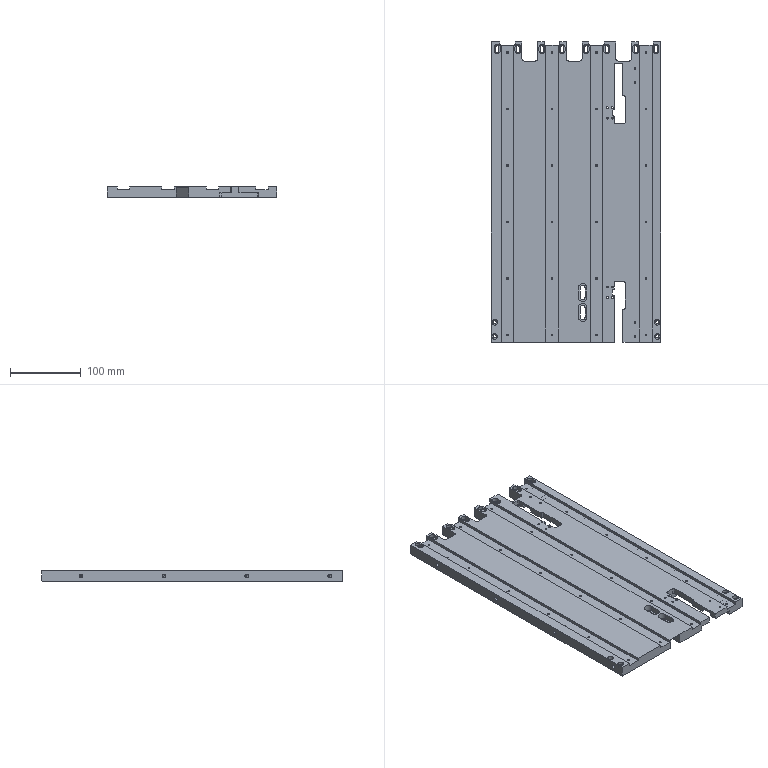Part | NX | features BREP 1 | 1 solid | 410 faces | box 240 x 425 x 15 mm | volume 1267639 mm3 | cylinder 182 | plane 162 | cone 66 | commonest cylinder face diameters 2.5 x72 4 x30 4.5 x24 8 x24 5 x18 6 x6